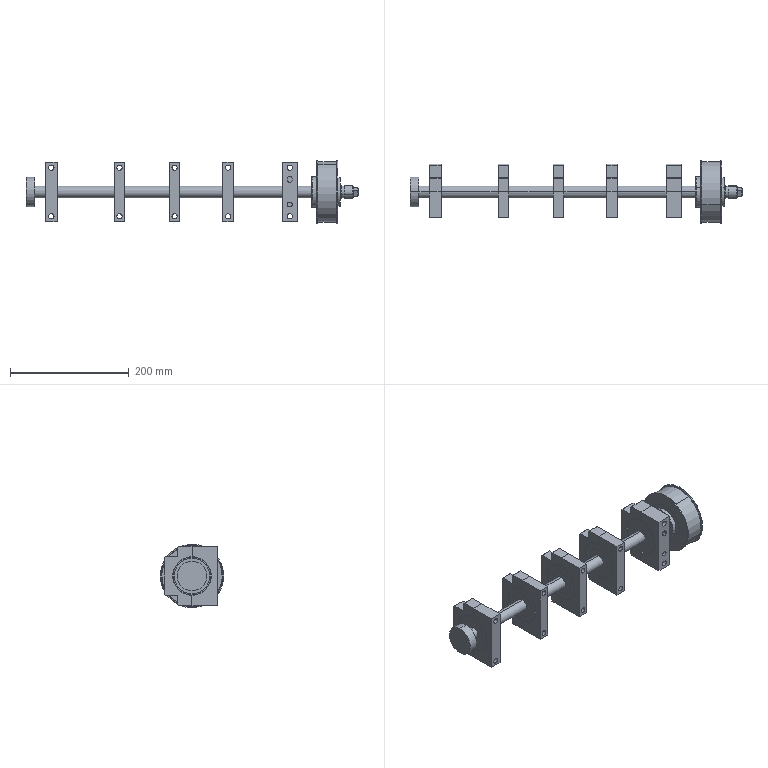Part | SolidWorks | 20 solids | 562 faces | box 559.6 x 107 x 107 mm | volume 1225428 mm3 | cylinder 264 | plane 232 | cone 46 | torus 10 | spline 10 | commonest cylinder face diameters 4 x40 9 x40 60 x20 65 x20 64 x18 20 x14